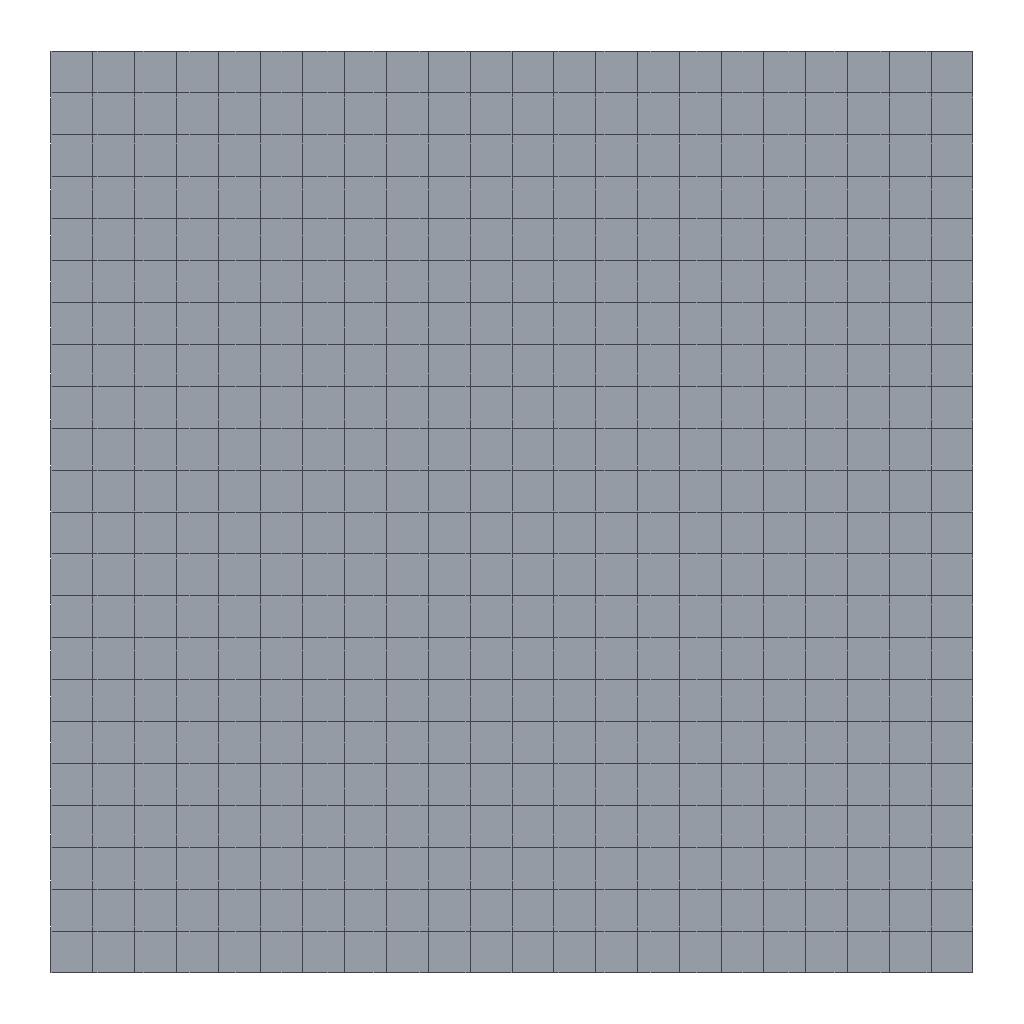Simulation study | abaqus
Set-up summary:
category,name,step,type,value,unit,region
solver,abaqus,,Abaqus/CAE 2024
units,mm-N-s-tonne (MPa),,inferred,E=193000 density=
analysis,Step-1,,static,time_period=1
mesh,nodes,,,529
mesh,elements,,,484
element_type,S4R,,,484
material,Material-1,,E,193000
material,Material-1,,nu,0.32
section,Material-1,,shell section,5,,_PickedSet2
load,Load-1,Step-1,pressure,1.22,,_PickedSurf8
bc,BC-1,Step-1,fixed,"[dofs=x,z n=2]",,_PickedSet4
bc,BC-2,Step-1,fixed,[dofs=z],,_PickedSet5
bc,BC-3,Step-1,fixed,"[dofs=y,z n=2]",,_PickedSet6
bc,BC-4,Step-1,fixed,[dofs=z],,_PickedSet7
Abaqus input file, long lists of numbers shortened:
*Heading
** Job name: deck Model name: Model-1
** Generated by: Abaqus/CAE 2024
*Preprint, echo=NO, model=NO, history=NO, contact=NO
**
** PARTS
**
*Part, name=Part-1
*Node
      1,         -40.,       216.75,           0.
      2,   -50.136,       216.75,           0.
** (527 more lines like these left out)
*Element, type=S4R
  1,   1,   2,  25,  24
  2,   2,   3,  26,  25
** (482 more lines like these left out)
*Nset, nset=_PickedSet2, internal, generate
   1,  529,    1
*Elset, elset=_PickedSet2, internal, generate
   1,  484,    1
** Section: Section-1
*Shell Section, elset=_PickedSet2, material=Material-1
5., 5
*End Part
**
**
** ASSEMBLY
**
*Assembly, name=Assembly
**
*Instance, name=Part-1-1, part=Part-1
        263.,         6.25,           0.
*End Instance
**
*Nset, nset=_PickedSet4, internal, instance=Part-1-1, generate
  23,  529,   23
*Elset, elset=_PickedSet4, internal, instance=Part-1-1, generate
  22,  484,   22
*Nset, nset=_PickedSet5, internal, instance=Part-1-1, generate
   1,  507,   23
*Elset, elset=_PickedSet5, internal, instance=Part-1-1, generate
   1,  463,   22
*Nset, nset=_PickedSet6, internal, instance=Part-1-1, generate
 507,  529,    1
*Elset, elset=_PickedSet6, internal, instance=Part-1-1, generate
 463,  484,    1
*Nset, nset=_PickedSet7, internal, instance=Part-1-1, generate
  1,  23,   1
*Elset, elset=_PickedSet7, internal, instance=Part-1-1, generate
  1,  22,   1
*Elset, elset=__PickedSurf8_SPOS, internal, instance=Part-1-1, generate
   1,  484,    1
*Surface, type=ELEMENT, name=_PickedSurf8, internal
__PickedSurf8_SPOS, SPOS
*End Assembly
**
** MATERIALS
**
*Material, name=Material-1
*Elastic
193000., 0.32
** ----------------------------------------------------------------
**
** STEP: Step-1
**
*Step, name=Step-1, nlgeom=NO
*Static
0.1, 1., 1e-05, 0.1
**
** BOUNDARY CONDITIONS
**
** Name: BC-1 Type: Displacement/Rotation
*Boundary
_PickedSet4, 1, 1
_PickedSet4, 3, 3
** Name: BC-2 Type: Displacement/Rotation
*Boundary
_PickedSet5, 3, 3
** Name: BC-3 Type: Displacement/Rotation
*Boundary
_PickedSet6, 2, 2
_PickedSet6, 3, 3
** Name: BC-4 Type: Displacement/Rotation
*Boundary
_PickedSet7, 3, 3
**
** LOADS
**
** Name: Load-1   Type: Pressure
*Dsload
_PickedSurf8, P, 1.22
**
** OUTPUT REQUESTS
**
*Restart, write, frequency=0
**
** FIELD OUTPUT: F-Output-1
**
*Output, field, variable=PRESELECT
**
** HISTORY OUTPUT: H-Output-1
**
*Output, history, variable=PRESELECT
*End Step
Results summary:
result,odb.job_status,,,JOB_STATUS_COMPLETED_SUCCESSFULLY,"consistent, unstated (Abaqus has no unit system)"
result,steps[0].procedure,Step-1,,*STATIC,"consistent, unstated (Abaqus has no unit system)"
result,steps[0].time_period,Step-1,,1,"consistent, unstated (Abaqus has no unit system)"
result,steps[0].n_frames,Step-1,,11,"consistent, unstated (Abaqus has no unit system)"
result,steps[0].last_frame.id,Step-1,,10,"consistent, unstated (Abaqus has no unit system)"
result,steps[0].last_frame.value,Step-1,,1,"consistent, unstated (Abaqus has no unit system)"
result,steps[0].last_frame.description,Step-1,,Increment     10: Step Time =    1.000,"consistent, unstated (Abaqus has no unit system)"
result,steps[0].completed,Step-1,,True,"consistent, unstated (Abaqus has no unit system)"
result,steps[0].max_U_magnitude,Step-1,,5.563,"consistent, unstated (Abaqus has no unit system)"
result,steps[0].max_S_mises,Step-1,,845.705,"consistent, unstated (Abaqus has no unit system)"
result,steps[0].RF_sum[1],Step-1,,5.85173e-14,"consistent, unstated (Abaqus has no unit system)"
result,steps[0].RF_sum[2],Step-1,,1.80057e-13,"consistent, unstated (Abaqus has no unit system)"
result,steps[0].RF_sum[3],Step-1,,60669.4,"consistent, unstated (Abaqus has no unit system)"